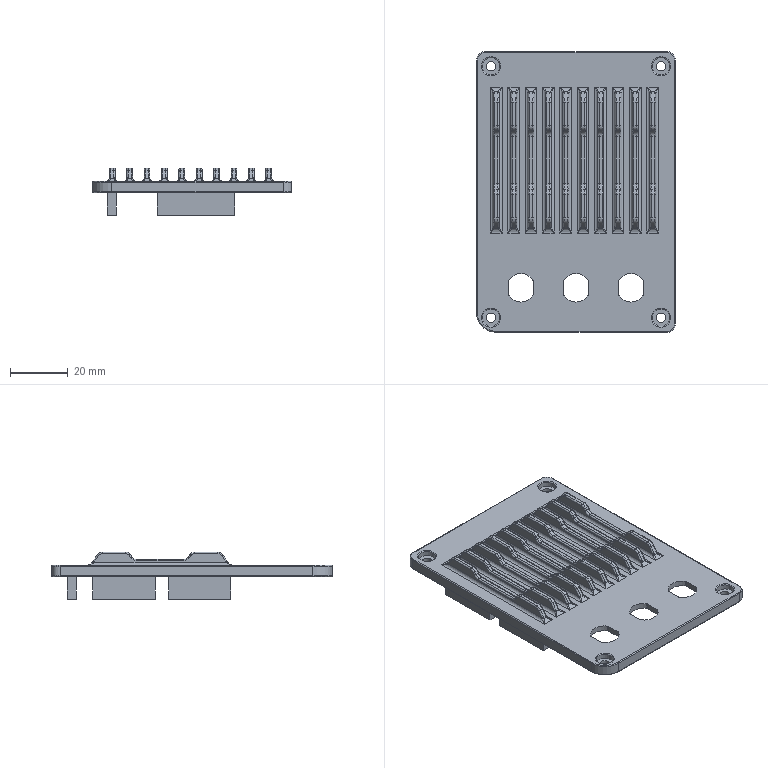NC program | NX | posted with a generic post | part box 68.665 x 96.782 x 16.5 mm
Lines 2053 to 2897 of 111885:
(PLANAR_MILL , TOOL : D3平刀)
N4080 T02 M6
N4082 G53
N4084 G17 G0 G90 X-38.291 Y1.421 S4500 M3
N4086 G43 Z20. H2
N4088 Z0.2
N4090 G94 G1 Y-15.043 Z0.056 F2000.
N4092 X-38.535 Y-15.636 Z0.051
N4094 X-38.987 Y-16.089 Z0.045
N4096 X-39.58 Y-16.332 Z0.04
N4098 X-43.302 Z0.007
N4100 X-43.895 Y-16.089 Z0.001
N4102 X-44.347 Y-15.636 Z-0.004
N4104 X-44.591 Y-15.044 Z-0.01
N4106 X-44.61 Y12.36 Z-0.249
N4108 X-44.368 Y12.95 Z-0.254
N4110 X-43.919 Y13.402 Z-0.26
N4112 X-43.33 Y13.648 Z-0.266
N4114 X-39.589 Y13.67 Z-0.298
N4116 X-38.993 Y13.428 Z-0.304
N4118 X-38.536 Y12.974 Z-0.309
N4120 X-38.291 Y12.379 Z-0.315
N4122 Y-15.043 Z-0.554
N4124 X-38.535 Y-15.636 Z-0.56
N4126 X-38.987 Y-16.089 Z-0.566
N4128 X-39.58 Y-16.332 Z-0.571
N4130 X-43.302 Z-0.604
N4132 X-43.895 Y-16.089 Z-0.609
N4134 X-44.347 Y-15.636 Z-0.615
N4136 X-44.591 Y-15.044 Z-0.62
N4138 X-44.61 Y12.36 Z-0.86
N4140 X-44.368 Y12.95 Z-0.865
N4142 X-43.919 Y13.402 Z-0.871
N4144 X-43.33 Y13.648 Z-0.876
N4146 X-39.589 Y13.67 Z-0.909
N4148 X-38.993 Y13.428 Z-0.914
N4150 X-38.536 Y12.974 Z-0.92
N4152 X-38.291 Y12.379 Z-0.926
N4154 Y-15.043 Z-1.165
N4156 X-38.535 Y-15.636 Z-1.171
N4158 X-38.987 Y-16.089 Z-1.176
N4160 X-39.58 Y-16.332 Z-1.182
N4162 X-43.302 Z-1.214
N4164 X-43.895 Y-16.089 Z-1.22
N4166 X-44.347 Y-15.636 Z-1.225
N4168 X-44.591 Y-15.044 Z-1.231
N4170 X-44.61 Y12.36 Z-1.47
N4172 X-44.368 Y12.95 Z-1.476
N4174 X-43.919 Y13.402 Z-1.481
N4176 X-43.33 Y13.648 Z-1.487
N4178 X-39.589 Y13.67 Z-1.52
N4180 X-38.993 Y13.428 Z-1.525
N4182 X-38.536 Y12.974 Z-1.531
N4184 X-38.291 Y12.379 Z-1.536
N4186 Y-15.043 Z-1.776
N4188 X-38.535 Y-15.636 Z-1.781
N4190 X-38.987 Y-16.089 Z-1.787
N4192 X-39.58 Y-16.332 Z-1.792
N4194 X-43.302 Z-1.825
N4196 X-43.895 Y-16.089 Z-1.831
N4198 X-44.347 Y-15.636 Z-1.836
N4200 X-44.591 Y-15.044 Z-1.842
N4202 X-44.61 Y12.36 Z-2.081
N4204 X-44.368 Y12.95 Z-2.086
N4206 X-43.919 Y13.402 Z-2.092
N4208 X-43.33 Y13.648 Z-2.098
N4210 X-39.589 Y13.67 Z-2.13
N4212 X-38.993 Y13.428 Z-2.136
N4214 X-38.536 Y12.974 Z-2.141
N4216 X-38.291 Y12.379 Z-2.147
N4218 Y-15.043 Z-2.386
N4220 X-38.535 Y-15.636 Z-2.392
N4222 X-38.987 Y-16.089 Z-2.398
N4224 X-39.58 Y-16.332 Z-2.403
N4226 X-43.302 Z-2.436
N4228 X-43.895 Y-16.089 Z-2.441
N4230 X-44.347 Y-15.636 Z-2.447
N4232 X-44.591 Y-15.044 Z-2.452
N4234 X-44.61 Y12.36 Z-2.692
N4236 X-44.368 Y12.95 Z-2.697
N4238 X-43.919 Y13.402 Z-2.703
N4240 X-43.33 Y13.648 Z-2.708
N4242 X-39.589 Y13.67 Z-2.741
N4244 X-38.993 Y13.428 Z-2.746
N4246 X-38.536 Y12.974 Z-2.752
N4248 X-38.291 Y12.379 Z-2.758
N4250 Y-15.043 Z-2.997
N4252 X-38.535 Y-15.636 Z-3.003
N4254 X-38.987 Y-16.089 Z-3.008
N4256 X-39.58 Y-16.332 Z-3.014
N4258 X-43.302 Z-3.046
N4260 X-43.895 Y-16.089 Z-3.052
N4262 X-44.347 Y-15.636 Z-3.057
N4264 X-44.591 Y-15.044 Z-3.063
N4266 X-44.61 Y12.36 Z-3.302
N4268 X-44.368 Y12.95 Z-3.308
N4270 X-43.919 Y13.402 Z-3.313
N4272 X-43.33 Y13.648 Z-3.319
N4274 X-39.589 Y13.67 Z-3.352
N4276 X-38.993 Y13.428 Z-3.357
N4278 X-38.536 Y12.974 Z-3.363
N4280 X-38.291 Y12.379 Z-3.368
N4282 Y-15.043 Z-3.608
N4284 X-38.535 Y-15.636 Z-3.613
N4286 X-38.987 Y-16.089 Z-3.619
N4288 X-39.58 Y-16.332 Z-3.624
N4290 X-43.302 Z-3.657
N4292 X-43.895 Y-16.089 Z-3.663
N4294 X-44.347 Y-15.636 Z-3.668
N4296 X-44.591 Y-15.044 Z-3.674
N4298 X-44.61 Y12.36 Z-3.913
N4300 X-44.368 Y12.95 Z-3.918
N4302 X-43.919 Y13.402 Z-3.924
N4304 X-43.33 Y13.648 Z-3.93
N4306 X-39.589 Y13.67 Z-3.962
N4308 X-38.993 Y13.428 Z-3.968
N4310 X-38.536 Y12.974 Z-3.973
N4312 X-38.291 Y12.379 Z-3.979
N4314 Y-15.043 Z-4.218
N4316 X-38.535 Y-15.636 Z-4.224
N4318 X-38.987 Y-16.089 Z-4.23
N4320 X-39.58 Y-16.332 Z-4.235
N4322 X-43.302 Z-4.268
N4324 X-43.895 Y-16.089 Z-4.273
N4326 X-44.347 Y-15.636 Z-4.279
N4328 X-44.591 Y-15.044 Z-4.284
N4330 X-44.61 Y12.36 Z-4.524
N4332 X-44.368 Y12.95 Z-4.529
N4334 X-43.919 Y13.402 Z-4.535
N4336 X-43.33 Y13.648 Z-4.54
N4338 X-39.589 Y13.67 Z-4.573
N4340 X-38.993 Y13.428 Z-4.579
N4342 X-38.536 Y12.974 Z-4.584
N4344 X-38.291 Y12.379 Z-4.59
N4346 Y-15.043 Z-4.829
N4348 X-38.535 Y-15.636 Z-4.835
N4350 X-38.987 Y-16.089 Z-4.84
N4352 X-39.58 Y-16.332 Z-4.846
N4354 X-43.302 Z-4.878
N4356 X-43.895 Y-16.089 Z-4.884
N4358 X-44.347 Y-15.636 Z-4.889
N4360 X-44.591 Y-15.044 Z-4.895
N4362 X-44.61 Y12.36 Z-5.134
N4364 X-44.368 Y12.95 Z-5.14
N4366 X-43.919 Y13.402 Z-5.145
N4368 X-43.33 Y13.648 Z-5.151
N4370 X-39.589 Y13.67 Z-5.184
N4372 X-38.993 Y13.428 Z-5.189
N4374 X-38.536 Y12.974 Z-5.195
N4376 X-38.291 Y12.379 Z-5.2
N4378 Y-15.043 Z-5.44
N4380 X-38.535 Y-15.636 Z-5.445
N4382 X-38.987 Y-16.089 Z-5.451
N4384 X-39.58 Y-16.332 Z-5.456
N4386 X-43.302 Z-5.489
N4388 X-43.895 Y-16.089 Z-5.495
N4390 X-44.347 Y-15.636 Z-5.5
N4392 X-44.591 Y-15.044 Z-5.506
N4394 X-44.61 Y12.36 Z-5.745
N4396 X-44.368 Y12.95 Z-5.75
N4398 X-43.919 Y13.402 Z-5.756
N4400 X-43.33 Y13.648 Z-5.762
N4402 X-39.589 Y13.67 Z-5.794
N4404 X-38.993 Y13.428 Z-5.8
N4406 X-38.536 Y12.974 Z-5.805
N4408 X-38.291 Y12.379 Z-5.811
N4410 Y-15.043 Z-6.05
N4412 X-38.535 Y-15.636 Z-6.056
N4414 X-38.987 Y-16.089 Z-6.062
N4416 X-39.58 Y-16.332 Z-6.067
N4418 X-43.302 Z-6.1
N4420 X-43.895 Y-16.089 Z-6.105
N4422 X-44.347 Y-15.636 Z-6.111
N4424 X-44.591 Y-15.044 Z-6.116
N4426 X-44.61 Y12.36 Z-6.356
N4428 X-44.368 Y12.95 Z-6.361
N4430 X-43.919 Y13.402 Z-6.367
N4432 X-43.33 Y13.648 Z-6.372
N4434 X-39.589 Y13.67 Z-6.405
N4436 X-38.993 Y13.428 Z-6.411
N4438 X-38.536 Y12.974 Z-6.416
N4440 X-38.291 Y12.379 Z-6.422
N4442 Y-15.043 Z-6.661
N4444 X-38.535 Y-15.636 Z-6.667
N4446 X-38.987 Y-16.089 Z-6.672
N4448 X-39.58 Y-16.332 Z-6.678
N4450 X-43.302 Z-6.71
N4452 X-43.895 Y-16.089 Z-6.716
N4454 X-44.347 Y-15.636 Z-6.721
N4456 X-44.591 Y-15.044 Z-6.727
N4458 X-44.61 Y12.36 Z-6.966
N4460 X-44.368 Y12.95 Z-6.972
N4462 X-43.919 Y13.402 Z-6.977
N4464 X-43.33 Y13.648 Z-6.983
N4466 X-39.589 Y13.67 Z-7.016
N4468 X-38.993 Y13.428 Z-7.021
N4470 X-38.536 Y12.974 Z-7.027
N4472 X-38.291 Y12.379 Z-7.032
N4474 Y-15.043 Z-7.272
N4476 X-38.535 Y-15.636 Z-7.277
N4478 X-38.987 Y-16.089 Z-7.283
N4480 X-39.58 Y-16.332 Z-7.288
N4482 X-43.302 Z-7.321
N4484 X-43.895 Y-16.089 Z-7.327
N4486 X-44.347 Y-15.636 Z-7.332
N4488 X-44.591 Y-15.044 Z-7.338
N4490 X-44.61 Y12.36 Z-7.577
N4492 X-44.368 Y12.95 Z-7.582
N4494 X-43.919 Y13.402 Z-7.588
N4496 X-43.33 Y13.648 Z-7.594
N4498 X-39.589 Y13.67 Z-7.626
N4500 X-38.993 Y13.428 Z-7.632
N4502 X-38.536 Y12.974 Z-7.637
N4504 X-38.291 Y12.379 Z-7.643
N4506 Y-15.043 Z-7.882
N4508 X-38.535 Y-15.636 Z-7.888
N4510 X-38.987 Y-16.089 Z-7.894
N4512 X-39.58 Y-16.332 Z-7.899
N4514 X-43.302 Z-7.932
N4516 X-43.895 Y-16.089 Z-7.937
N4518 X-44.347 Y-15.636 Z-7.943
N4520 X-44.591 Y-15.044 Z-7.948
N4522 X-44.61 Y12.36 Z-8.188
N4524 X-44.368 Y12.95 Z-8.193
N4526 X-43.919 Y13.402 Z-8.199
N4528 X-43.33 Y13.648 Z-8.204
N4530 X-39.589 Y13.67 Z-8.237
N4532 X-38.993 Y13.428 Z-8.243
N4534 X-38.536 Y12.974 Z-8.248
N4536 X-38.291 Y12.379 Z-8.254
N4538 Y-15.043 Z-8.493
N4540 X-38.535 Y-15.636 Z-8.499
N4542 X-38.987 Y-16.089 Z-8.504
N4544 X-39.58 Y-16.332 Z-8.51
N4546 X-43.302 Z-8.542
N4548 X-43.895 Y-16.089 Z-8.548
N4550 X-44.347 Y-15.636 Z-8.553
N4552 X-44.591 Y-15.044 Z-8.559
N4554 X-44.61 Y12.36 Z-8.798
N4556 X-44.368 Y12.95 Z-8.804
N4558 X-43.919 Y13.402 Z-8.809
N4560 X-43.33 Y13.648 Z-8.815
N4562 X-39.589 Y13.67 Z-8.848
N4564 X-38.993 Y13.428 Z-8.853
N4566 X-38.536 Y12.974 Z-8.859
N4568 X-38.291 Y12.379 Z-8.864
N4570 Y-15.043 Z-9.104
N4572 X-38.535 Y-15.636 Z-9.109
N4574 X-38.987 Y-16.089 Z-9.115
N4576 X-39.58 Y-16.332 Z-9.121
N4578 X-43.302 Z-9.153
N4580 X-43.895 Y-16.089 Z-9.159
N4582 X-44.347 Y-15.636 Z-9.164
N4584 X-44.591 Y-15.044 Z-9.17
N4586 X-44.61 Y12.36 Z-9.409
N4588 X-44.368 Y12.95 Z-9.414
N4590 X-43.919 Y13.402 Z-9.42
N4592 X-43.33 Y13.648 Z-9.426
N4594 X-39.589 Y13.67 Z-9.458
N4596 X-38.993 Y13.428 Z-9.464
N4598 X-38.536 Y12.974 Z-9.469
N4600 X-38.291 Y12.379 Z-9.475
N4602 Y-15.043 Z-9.714
N4604 X-38.535 Y-15.636 Z-9.72
N4606 X-38.987 Y-16.089 Z-9.726
N4608 X-39.58 Y-16.332 Z-9.731
N4610 X-43.302 Z-9.764
N4612 X-43.895 Y-16.089 Z-9.769
N4614 X-44.347 Y-15.636 Z-9.775
N4616 X-44.591 Y-15.044 Z-9.78
N4618 X-44.6 Y-1.342 Z-9.9
N4620 X-44.609 Y12.048
N4622 G2 X-43.019 Y13.65 R1.6
N4624 G1 X-39.901 Y13.668
N4626 G2 X-38.291 Y12.068 R1.6
N4628 G1 Y-14.732
N4630 G2 X-39.891 Y-16.332 R1.6
N4632 G1 X-42.991
N4634 G2 X-44.591 Y-14.733 R1.6
N4636 G1 X-44.6 Y-1.342
N4638 Z-9.7
N4640 G0 Z20.
N4642 X-23.934 Y24.568
N4644 Z0.2
N4646 G1 X-34.502 Z0.108
N4648 X-35.095 Y24.811 Z0.102
N4650 X-35.548 Y25.264 Z0.097
N4652 X-35.791 Y25.857 Z0.091
N4654 Y29.597 Z0.058
N4656 X-35.548 Y30.19 Z0.053
N4658 X-35.095 Y30.643 Z0.047
N4660 X-34.502 Y30.886 Z0.042
N4662 X-12.398 Z-0.151
N4664 X-11.806 Y30.643 Z-0.157
N4666 X-11.353 Y30.19 Z-0.162
N4668 X-11.109 Y29.597 Z-0.168
N4670 Y25.857 Z-0.201
N4672 X-11.353 Y25.264 Z-0.206
N4674 X-11.806 Y24.811 Z-0.212
N4676 X-12.398 Y24.568 Z-0.217
N4678 X-34.502 Z-0.41
N4680 X-35.095 Y24.811 Z-0.416
N4682 X-35.548 Y25.264 Z-0.422
N4684 X-35.791 Y25.857 Z-0.427
N4686 Y29.597 Z-0.46
N4688 X-35.548 Y30.19 Z-0.465
N4690 X-35.095 Y30.643 Z-0.471
N4692 X-34.502 Y30.886 Z-0.477
N4694 X-12.398 Z-0.669
N4696 X-11.806 Y30.643 Z-0.675
N4698 X-11.353 Y30.19 Z-0.681
N4700 X-11.109 Y29.597 Z-0.686
N4702 Y25.857 Z-0.719
N4704 X-11.353 Y25.264 Z-0.724
N4706 X-11.806 Y24.811 Z-0.73
N4708 X-12.398 Y24.568 Z-0.736
N4710 X-34.502 Z-0.929
N4712 X-35.095 Y24.811 Z-0.934
N4714 X-35.548 Y25.264 Z-0.94
N4716 X-35.791 Y25.857 Z-0.945
N4718 Y29.597 Z-0.978
N4720 X-35.548 Y30.19 Z-0.984
N4722 X-35.095 Y30.643 Z-0.989
N4724 X-34.502 Y30.886 Z-0.995
N4726 X-12.398 Z-1.188
N4728 X-11.806 Y30.643 Z-1.193
N4730 X-11.353 Y30.19 Z-1.199
N4732 X-11.109 Y29.597 Z-1.204
N4734 Y25.857 Z-1.237
N4736 X-11.353 Y25.264 Z-1.243
N4738 X-11.806 Y24.811 Z-1.248
N4740 X-12.398 Y24.568 Z-1.254
N4742 X-34.502 Z-1.447
N4744 X-35.095 Y24.811 Z-1.452
N4746 X-35.548 Y25.264 Z-1.458
N4748 X-35.791 Y25.857 Z-1.463
N4750 Y29.597 Z-1.496
N4752 X-35.548 Y30.19 Z-1.502
N4754 X-35.095 Y30.643 Z-1.507
N4756 X-34.502 Y30.886 Z-1.513
N4758 X-12.398 Z-1.706
N4760 X-11.806 Y30.643 Z-1.711
N4762 X-11.353 Y30.19 Z-1.717
N4764 X-11.109 Y29.597 Z-1.723
N4766 Y25.857 Z-1.755
N4768 X-11.353 Y25.264 Z-1.761
N4770 X-11.806 Y24.811 Z-1.766
N4772 X-12.398 Y24.568 Z-1.772
N4774 X-34.502 Z-1.965
N4776 X-35.095 Y24.811 Z-1.97
N4778 X-35.548 Y25.264 Z-1.976
N4780 X-35.791 Y25.857 Z-1.982
N4782 Y29.597 Z-2.014
N4784 X-35.548 Y30.19 Z-2.02
N4786 X-35.095 Y30.643 Z-2.025
N4788 X-34.502 Y30.886 Z-2.031
N4790 X-12.398 Z-2.224
N4792 X-11.806 Y30.643 Z-2.23
N4794 X-11.353 Y30.19 Z-2.235
N4796 X-11.109 Y29.597 Z-2.241
N4798 Y25.857 Z-2.273
N4800 X-11.353 Y25.264 Z-2.279
N4802 X-11.806 Y24.811 Z-2.285
N4804 X-12.398 Y24.568 Z-2.29
N4806 X-34.502 Z-2.483
N4808 X-35.095 Y24.811 Z-2.489
N4810 X-35.548 Y25.264 Z-2.494
N4812 X-35.791 Y25.857 Z-2.5
N4814 Y29.597 Z-2.532
N4816 X-35.548 Y30.19 Z-2.538
N4818 X-35.095 Y30.643 Z-2.544
N4820 X-34.502 Y30.886 Z-2.549
N4822 X-12.398 Z-2.742
N4824 X-11.806 Y30.643 Z-2.748
N4826 X-11.353 Y30.19 Z-2.753
N4828 X-11.109 Y29.597 Z-2.759
N4830 Y25.857 Z-2.792
N4832 X-11.353 Y25.264 Z-2.797
N4834 X-11.806 Y24.811 Z-2.803
N4836 X-12.398 Y24.568 Z-2.808
N4838 X-34.502 Z-3.001
N4840 X-35.095 Y24.811 Z-3.007
N4842 X-35.548 Y25.264 Z-3.012
N4844 X-35.791 Y25.857 Z-3.018
N4846 Y29.597 Z-3.051
N4848 X-35.548 Y30.19 Z-3.056
N4850 X-35.095 Y30.643 Z-3.062
N4852 X-34.502 Y30.886 Z-3.067
N4854 X-12.398 Z-3.26
N4856 X-11.806 Y30.643 Z-3.266
N4858 X-11.353 Y30.19 Z-3.271
N4860 X-11.109 Y29.597 Z-3.277
N4862 Y25.857 Z-3.31
N4864 X-11.353 Y25.264 Z-3.315
N4866 X-11.806 Y24.811 Z-3.321
N4868 X-12.398 Y24.568 Z-3.326
N4870 X-34.502 Z-3.519
N4872 X-35.095 Y24.811 Z-3.525
N4874 X-35.548 Y25.264 Z-3.531
N4876 X-35.791 Y25.857 Z-3.536
N4878 Y29.597 Z-3.569
N4880 X-35.548 Y30.19 Z-3.574
N4882 X-35.095 Y30.643 Z-3.58
N4884 X-34.502 Y30.886 Z-3.586
N4886 X-12.398 Z-3.778
N4888 X-11.806 Y30.643 Z-3.784
N4890 X-11.353 Y30.19 Z-3.79
N4892 X-11.109 Y29.597 Z-3.795
N4894 Y25.857 Z-3.828
N4896 X-11.353 Y25.264 Z-3.833
N4898 X-11.806 Y24.811 Z-3.839
N4900 X-12.398 Y24.568 Z-3.845
N4902 X-34.502 Z-4.038
N4904 X-35.095 Y24.811 Z-4.043
N4906 X-35.548 Y25.264 Z-4.049
N4908 X-35.791 Y25.857 Z-4.054
N4910 Y29.597 Z-4.087
N4912 X-35.548 Y30.19 Z-4.093
N4914 X-35.095 Y30.643 Z-4.098
N4916 X-34.502 Y30.886 Z-4.104
N4918 X-12.398 Z-4.297
N4920 X-11.806 Y30.643 Z-4.302
N4922 X-11.353 Y30.19 Z-4.308
N4924 X-11.109 Y29.597 Z-4.313
N4926 Y25.857 Z-4.346
N4928 X-11.353 Y25.264 Z-4.352
N4930 X-11.806 Y24.811 Z-4.357
N4932 X-12.398 Y24.568 Z-4.363
N4934 X-34.502 Z-4.556
N4936 X-35.095 Y24.811 Z-4.561
N4938 X-35.548 Y25.264 Z-4.567
N4940 X-35.791 Y25.857 Z-4.572
N4942 Y29.597 Z-4.605
N4944 X-35.548 Y30.19 Z-4.611
N4946 X-35.095 Y30.643 Z-4.616
N4948 X-34.502 Y30.886 Z-4.622
N4950 X-12.398 Z-4.815
N4952 X-11.806 Y30.643 Z-4.82
N4954 X-11.353 Y30.19 Z-4.826
N4956 X-11.109 Y29.597 Z-4.832
N4958 Y25.857 Z-4.864
N4960 X-11.353 Y25.264 Z-4.87
N4962 X-11.806 Y24.811 Z-4.875
N4964 X-12.398 Y24.568 Z-4.881
N4966 X-34.502 Z-5.074
N4968 X-35.095 Y24.811 Z-5.079
N4970 X-35.548 Y25.264 Z-5.085
N4972 X-35.791 Y25.857 Z-5.091
N4974 Y29.597 Z-5.123
N4976 X-35.548 Y30.19 Z-5.129
N4978 X-35.095 Y30.643 Z-5.134
N4980 X-34.502 Y30.886 Z-5.14
N4982 X-12.398 Z-5.333
N4984 X-11.806 Y30.643 Z-5.339
N4986 X-11.353 Y30.19 Z-5.344
N4988 X-11.109 Y29.597 Z-5.35
N4990 Y25.857 Z-5.382
N4992 X-11.353 Y25.264 Z-5.388
N4994 X-11.806 Y24.811 Z-5.394
N4996 X-12.398 Y24.568 Z-5.399
N4998 X-34.502 Z-5.592
N5000 X-35.095 Y24.811 Z-5.598
N5002 X-35.548 Y25.264 Z-5.603
N5004 X-35.791 Y25.857 Z-5.609
N5006 Y29.597 Z-5.641
N5008 X-35.548 Y30.19 Z-5.647
N5010 X-35.095 Y30.643 Z-5.653
N5012 X-34.502 Y30.886 Z-5.658
N5014 X-12.398 Z-5.851
N5016 X-11.806 Y30.643 Z-5.857
N5018 X-11.353 Y30.19 Z-5.862
N5020 X-11.109 Y29.597 Z-5.868
N5022 Y25.857 Z-5.901
N5024 X-11.353 Y25.264 Z-5.906
N5026 X-11.806 Y24.811 Z-5.912
N5028 X-12.398 Y24.568 Z-5.917
N5030 X-34.502 Z-6.11
N5032 X-35.095 Y24.811 Z-6.116
N5034 X-35.548 Y25.264 Z-6.121
N5036 X-35.791 Y25.857 Z-6.127
N5038 Y29.597 Z-6.16
N5040 X-35.548 Y30.19 Z-6.165
N5042 X-35.095 Y30.643 Z-6.171
N5044 X-34.502 Y30.886 Z-6.176
N5046 X-12.398 Z-6.369
N5048 X-11.806 Y30.643 Z-6.375
N5050 X-11.353 Y30.19 Z-6.38
N5052 X-11.109 Y29.597 Z-6.386
N5054 Y25.857 Z-6.419
N5056 X-11.353 Y25.264 Z-6.424
N5058 X-11.806 Y24.811 Z-6.43
N5060 X-12.398 Y24.568 Z-6.435
N5062 X-34.502 Z-6.628
N5064 X-35.095 Y24.811 Z-6.634
N5066 X-35.548 Y25.264 Z-6.64
N5068 X-35.791 Y25.857 Z-6.645
N5070 Y29.597 Z-6.678
N5072 X-35.548 Y30.19 Z-6.683
N5074 X-35.095 Y30.643 Z-6.689
N5076 X-34.502 Y30.886 Z-6.695
N5078 X-12.398 Z-6.887
N5080 X-11.806 Y30.643 Z-6.893
N5082 X-11.353 Y30.19 Z-6.899
N5084 X-11.109 Y29.597 Z-6.904
N5086 Y25.857 Z-6.937
N5088 X-11.353 Y25.264 Z-6.942
N5090 X-11.806 Y24.811 Z-6.948
N5092 X-12.398 Y24.568 Z-6.954
N5094 X-34.502 Z-7.147
N5096 X-35.095 Y24.811 Z-7.152
N5098 X-35.548 Y25.264 Z-7.158
N5100 X-35.791 Y25.857 Z-7.163
N5102 Y29.597 Z-7.196
N5104 X-35.548 Y30.19 Z-7.202
N5106 X-35.095 Y30.643 Z-7.207
N5108 X-34.502 Y30.886 Z-7.213
N5110 X-12.398 Z-7.406
N5112 X-11.806 Y30.643 Z-7.411
N5114 X-11.353 Y30.19 Z-7.417
N5116 X-11.109 Y29.597 Z-7.422
N5118 Y25.857 Z-7.455
N5120 X-11.353 Y25.264 Z-7.461
N5122 X-11.806 Y24.811 Z-7.466
N5124 X-12.398 Y24.568 Z-7.472
N5126 X-34.502 Z-7.665
N5128 X-35.095 Y24.811 Z-7.67
N5130 X-35.548 Y25.264 Z-7.676
N5132 X-35.791 Y25.857 Z-7.681
N5134 Y29.597 Z-7.714
N5136 X-35.548 Y30.19 Z-7.72
N5138 X-35.095 Y30.643 Z-7.725
N5140 X-34.502 Y30.886 Z-7.731
N5142 X-12.398 Z-7.924
N5144 X-11.806 Y30.643 Z-7.929
N5146 X-11.353 Y30.19 Z-7.935
N5148 X-11.109 Y29.597 Z-7.941
N5150 Y25.857 Z-7.973
N5152 X-11.353 Y25.264 Z-7.979
N5154 X-11.806 Y24.811 Z-7.984
N5156 X-12.398 Y24.568 Z-7.99
N5158 X-34.502 Z-8.183
N5160 X-35.095 Y24.811 Z-8.188
N5162 X-35.548 Y25.264 Z-8.194
N5164 X-35.791 Y25.857 Z-8.2
N5166 Y29.597 Z-8.232
N5168 X-35.548 Y30.19 Z-8.238
N5170 X-35.095 Y30.643 Z-8.243
N5172 X-34.502 Y30.886 Z-8.249
N5174 X-12.398 Z-8.442
N5176 X-11.806 Y30.643 Z-8.448
N5178 X-11.353 Y30.19 Z-8.453
N5180 X-11.109 Y29.597 Z-8.459
N5182 Y25.857 Z-8.491
N5184 X-11.353 Y25.264 Z-8.497
N5186 X-11.806 Y24.811 Z-8.503
N5188 X-12.398 Y24.568 Z-8.508
N5190 X-34.502 Z-8.701
N5192 X-35.095 Y24.811 Z-8.707
N5194 X-35.548 Y25.264 Z-8.712
N5196 X-35.791 Y25.857 Z-8.718
N5198 Y29.597 Z-8.75
N5200 X-35.548 Y30.19 Z-8.756
N5202 X-35.095 Y30.643 Z-8.762
N5204 X-34.502 Y30.886 Z-8.767
N5206 X-12.398 Z-8.96
N5208 X-11.806 Y30.643 Z-8.966
N5210 X-11.353 Y30.19 Z-8.971
N5212 X-11.109 Y29.597 Z-8.977
N5214 Y25.857 Z-9.01
N5216 X-11.353 Y25.264 Z-9.015
N5218 X-11.806 Y24.811 Z-9.021
N5220 X-12.398 Y24.568 Z-9.026
N5222 X-34.502 Z-9.219
N5224 X-35.095 Y24.811 Z-9.225
N5226 X-35.548 Y25.264 Z-9.23
N5228 X-35.791 Y25.857 Z-9.236
N5230 Y29.597 Z-9.269
N5232 X-35.548 Y30.19 Z-9.274
N5234 X-35.095 Y30.643 Z-9.28
N5236 X-34.502 Y30.886 Z-9.285
N5238 X-12.398 Z-9.478
N5240 X-11.806 Y30.643 Z-9.484
N5242 X-11.353 Y30.19 Z-9.489
N5244 X-11.109 Y29.597 Z-9.495
N5246 Y25.857 Z-9.528
N5248 X-11.353 Y25.264 Z-9.533
N5250 X-11.806 Y24.811 Z-9.539
N5252 X-12.398 Y24.568 Z-9.544
N5254 X-34.502 Z-9.737
N5256 X-35.095 Y24.811 Z-9.743
N5258 X-35.548 Y25.264 Z-9.749
N5260 X-35.791 Y25.857 Z-9.754
N5262 Y29.597 Z-9.787
N5264 X-35.548 Y30.19 Z-9.792
N5266 X-35.095 Y30.643 Z-9.798
N5268 X-34.502 Y30.886 Z-9.804
N5270 X-23.45 Z-9.9
N5272 X-12.709
N5274 G2 X-11.109 Y29.286 R1.6
N5276 G1 Y26.168
N5278 G2 X-12.709 Y24.568 R1.6
N5280 G1 X-34.191
N5282 G2 X-35.791 Y26.168 R1.6
N5284 G1 Y29.286
N5286 G2 X-34.191 Y30.886 R1.6
N5288 G1 X-23.45
N5290 Z-9.7
N5292 G0 Z20.
N5294 X2.184 Y24.568
N5296 Z0.2
N5298 G1 X-8.384 Z0.108
N5300 X-8.977 Y24.811 Z0.102
N5302 X-9.429 Y25.264 Z0.097
N5304 X-9.673 Y25.857 Z0.091
N5306 Y29.597 Z0.058
N5308 X-9.429 Y30.19 Z0.053
N5310 X-8.977 Y30.643 Z0.047
N5312 X-8.384 Y30.886 Z0.042
N5314 X13.72 Z-0.151
N5316 X14.313 Y30.643 Z-0.157
N5318 X14.765 Y30.19 Z-0.162
N5320 X15.009 Y29.597 Z-0.168
N5322 Y25.857 Z-0.201
N5324 X14.765 Y25.264 Z-0.206
N5326 X14.313 Y24.811 Z-0.212
N5328 X13.72 Y24.568 Z-0.217
N5330 X-8.384 Z-0.41
N5332 X-8.977 Y24.811 Z-0.416
N5334 X-9.429 Y25.264 Z-0.422
N5336 X-9.673 Y25.857 Z-0.427
N5338 Y29.597 Z-0.46
N5340 X-9.429 Y30.19 Z-0.465
N5342 X-8.977 Y30.643 Z-0.471
N5344 X-8.384 Y30.886 Z-0.477
N5346 X13.72 Z-0.669
N5348 X14.313 Y30.643 Z-0.675
N5350 X14.765 Y30.19 Z-0.681
N5352 X15.009 Y29.597 Z-0.686
N5354 Y25.857 Z-0.719
N5356 X14.765 Y25.264 Z-0.724
N5358 X14.313 Y24.811 Z-0.73
N5360 X13.72 Y24.568 Z-0.736
N5362 X-8.384 Z-0.929
N5364 X-8.977 Y24.811 Z-0.934
N5366 X-9.429 Y25.264 Z-0.94
N5368 X-9.673 Y25.857 Z-0.945
N5370 Y29.597 Z-0.978
N5372 X-9.429 Y30.19 Z-0.984
N5374 X-8.977 Y30.643 Z-0.989
N5376 X-8.384 Y30.886 Z-0.995
N5378 X13.72 Z-1.188
N5380 X14.313 Y30.643 Z-1.193
N5382 X14.765 Y30.19 Z-1.199
N5384 X15.009 Y29.597 Z-1.204
N5386 Y25.857 Z-1.237
N5388 X14.765 Y25.264 Z-1.243
N5390 X14.313 Y24.811 Z-1.248
N5392 X13.72 Y24.568 Z-1.254
N5394 X-8.384 Z-1.447
N5396 X-8.977 Y24.811 Z-1.452
N5398 X-9.429 Y25.264 Z-1.458
N5400 X-9.673 Y25.857 Z-1.463
N5402 Y29.597 Z-1.496
N5404 X-9.429 Y30.19 Z-1.502
N5406 X-8.977 Y30.643 Z-1.507
N5408 X-8.384 Y30.886 Z-1.513
N5410 X13.72 Z-1.706
N5412 X14.313 Y30.643 Z-1.711
N5414 X14.765 Y30.19 Z-1.717
N5416 X15.009 Y29.597 Z-1.723
N5418 Y25.857 Z-1.755
N5420 X14.765 Y25.264 Z-1.761
N5422 X14.313 Y24.811 Z-1.766
N5424 X13.72 Y24.568 Z-1.772
N5426 X-8.384 Z-1.965
N5428 X-8.977 Y24.811 Z-1.97
N5430 X-9.429 Y25.264 Z-1.976
N5432 X-9.673 Y25.857 Z-1.982
N5434 Y29.597 Z-2.014
N5436 X-9.429 Y30.19 Z-2.02
N5438 X-8.977 Y30.643 Z-2.025
N5440 X-8.384 Y30.886 Z-2.031
N5442 X13.72 Z-2.224
N5444 X14.313 Y30.643 Z-2.23
N5446 X14.765 Y30.19 Z-2.235
N5448 X15.009 Y29.597 Z-2.241
N5450 Y25.857 Z-2.273
N5452 X14.765 Y25.264 Z-2.279
N5454 X14.313 Y24.811 Z-2.285
N5456 X13.72 Y24.568 Z-2.29
N5458 X-8.384 Z-2.483
N5460 X-8.977 Y24.811 Z-2.489
N5462 X-9.429 Y25.264 Z-2.494
N5464 X-9.673 Y25.857 Z-2.5
N5466 Y29.597 Z-2.532
N5468 X-9.429 Y30.19 Z-2.538
N5470 X-8.977 Y30.643 Z-2.544
N5472 X-8.384 Y30.886 Z-2.549
N5474 X13.72 Z-2.742
N5476 X14.313 Y30.643 Z-2.748
N5478 X14.765 Y30.19 Z-2.753
N5480 X15.009 Y29.597 Z-2.759
N5482 Y25.857 Z-2.792
N5484 X14.765 Y25.264 Z-2.797
N5486 X14.313 Y24.811 Z-2.803
N5488 X13.72 Y24.568 Z-2.808
N5490 X-8.384 Z-3.001
N5492 X-8.977 Y24.811 Z-3.007
N5494 X-9.429 Y25.264 Z-3.012
N5496 X-9.673 Y25.857 Z-3.018
N5498 Y29.597 Z-3.051
N5500 X-9.429 Y30.19 Z-3.056
N5502 X-8.977 Y30.643 Z-3.062
N5504 X-8.384 Y30.886 Z-3.067
N5506 X13.72 Z-3.26
N5508 X14.313 Y30.643 Z-3.266
N5510 X14.765 Y30.19 Z-3.271
N5512 X15.009 Y29.597 Z-3.277
N5514 Y25.857 Z-3.31
N5516 X14.765 Y25.264 Z-3.315
N5518 X14.313 Y24.811 Z-3.321
N5520 X13.72 Y24.568 Z-3.326
N5522 X-8.384 Z-3.519
N5524 X-8.977 Y24.811 Z-3.525
N5526 X-9.429 Y25.264 Z-3.531
N5528 X-9.673 Y25.857 Z-3.536
N5530 Y29.597 Z-3.569
N5532 X-9.429 Y30.19 Z-3.574
N5534 X-8.977 Y30.643 Z-3.58
N5536 X-8.384 Y30.886 Z-3.586
N5538 X13.72 Z-3.778
N5540 X14.313 Y30.643 Z-3.784
N5542 X14.765 Y30.19 Z-3.79
N5544 X15.009 Y29.597 Z-3.795
N5546 Y25.857 Z-3.828
N5548 X14.765 Y25.264 Z-3.833
N5550 X14.313 Y24.811 Z-3.839
N5552 X13.72 Y24.568 Z-3.845
N5554 X-8.384 Z-4.038
N5556 X-8.977 Y24.811 Z-4.043
N5558 X-9.429 Y25.264 Z-4.049
N5560 X-9.673 Y25.857 Z-4.054
N5562 Y29.597 Z-4.087
N5564 X-9.429 Y30.19 Z-4.093
N5566 X-8.977 Y30.643 Z-4.098
N5568 X-8.384 Y30.886 Z-4.104
N5570 X13.72 Z-4.297
N5572 X14.313 Y30.643 Z-4.302
N5574 X14.765 Y30.19 Z-4.308
N5576 X15.009 Y29.597 Z-4.313
N5578 Y25.857 Z-4.346
N5580 X14.765 Y25.264 Z-4.352
N5582 X14.313 Y24.811 Z-4.357
N5584 X13.72 Y24.568 Z-4.363
N5586 X-8.384 Z-4.556
N5588 X-8.977 Y24.811 Z-4.561
N5590 X-9.429 Y25.264 Z-4.567
N5592 X-9.673 Y25.857 Z-4.572
N5594 Y29.597 Z-4.605
N5596 X-9.429 Y30.19 Z-4.611
N5598 X-8.977 Y30.643 Z-4.616
N5600 X-8.384 Y30.886 Z-4.622
N5602 X13.72 Z-4.815
N5604 X14.313 Y30.643 Z-4.82
N5606 X14.765 Y30.19 Z-4.826
N5608 X15.009 Y29.597 Z-4.832
N5610 Y25.857 Z-4.864
N5612 X14.765 Y25.264 Z-4.87
N5614 X14.313 Y24.811 Z-4.875
N5616 X13.72 Y24.568 Z-4.881
N5618 X-8.384 Z-5.074
N5620 X-8.977 Y24.811 Z-5.079
N5622 X-9.429 Y25.264 Z-5.085
N5624 X-9.673 Y25.857 Z-5.091
N5626 Y29.597 Z-5.123
N5628 X-9.429 Y30.19 Z-5.129
N5630 X-8.977 Y30.643 Z-5.134
N5632 X-8.384 Y30.886 Z-5.14
N5634 X13.72 Z-5.333
N5636 X14.313 Y30.643 Z-5.339
N5638 X14.765 Y30.19 Z-5.344
N5640 X15.009 Y29.597 Z-5.35
N5642 Y25.857 Z-5.382
N5644 X14.765 Y25.264 Z-5.388
N5646 X14.313 Y24.811 Z-5.394
N5648 X13.72 Y24.568 Z-5.399
N5650 X-8.384 Z-5.592
N5652 X-8.977 Y24.811 Z-5.598
N5654 X-9.429 Y25.264 Z-5.603
N5656 X-9.673 Y25.857 Z-5.609
N5658 Y29.597 Z-5.641
N5660 X-9.429 Y30.19 Z-5.647
N5662 X-8.977 Y30.643 Z-5.653
N5664 X-8.384 Y30.886 Z-5.658
N5666 X13.72 Z-5.851
N5668 X14.313 Y30.643 Z-5.857
N5670 X14.765 Y30.19 Z-5.862
N5672 X15.009 Y29.597 Z-5.868
N5674 Y25.857 Z-5.901
N5676 X14.765 Y25.264 Z-5.906
N5678 X14.313 Y24.811 Z-5.912
N5680 X13.72 Y24.568 Z-5.917
N5682 X-8.384 Z-6.11
N5684 X-8.977 Y24.811 Z-6.116
N5686 X-9.429 Y25.264 Z-6.121
N5688 X-9.673 Y25.857 Z-6.127
N5690 Y29.597 Z-6.16
N5692 X-9.429 Y30.19 Z-6.165
N5694 X-8.977 Y30.643 Z-6.171
N5696 X-8.384 Y30.886 Z-6.176
N5698 X13.72 Z-6.369
N5700 X14.313 Y30.643 Z-6.375
N5702 X14.765 Y30.19 Z-6.38
N5704 X15.009 Y29.597 Z-6.386
N5706 Y25.857 Z-6.419
N5708 X14.765 Y25.264 Z-6.424
N5710 X14.313 Y24.811 Z-6.43
N5712 X13.72 Y24.568 Z-6.435
N5714 X-8.384 Z-6.628
N5716 X-8.977 Y24.811 Z-6.634
N5718 X-9.429 Y25.264 Z-6.64
N5720 X-9.673 Y25.857 Z-6.645
N5722 Y29.597 Z-6.678
N5724 X-9.429 Y30.19 Z-6.683
N5726 X-8.977 Y30.643 Z-6.689
N5728 X-8.384 Y30.886 Z-6.695
N5730 X13.72 Z-6.887
N5732 X14.313 Y30.643 Z-6.893
N5734 X14.765 Y30.19 Z-6.899
N5736 X15.009 Y29.597 Z-6.904
N5738 Y25.857 Z-6.937
N5740 X14.765 Y25.264 Z-6.942
N5742 X14.313 Y24.811 Z-6.948
N5744 X13.72 Y24.568 Z-6.954
N5746 X-8.384 Z-7.147
N5748 X-8.977 Y24.811 Z-7.152
N5750 X-9.429 Y25.264 Z-7.158
N5752 X-9.673 Y25.857 Z-7.163
N5754 Y29.597 Z-7.196
N5756 X-9.429 Y30.19 Z-7.202
N5758 X-8.977 Y30.643 Z-7.207
N5760 X-8.384 Y30.886 Z-7.213
N5762 X13.72 Z-7.406